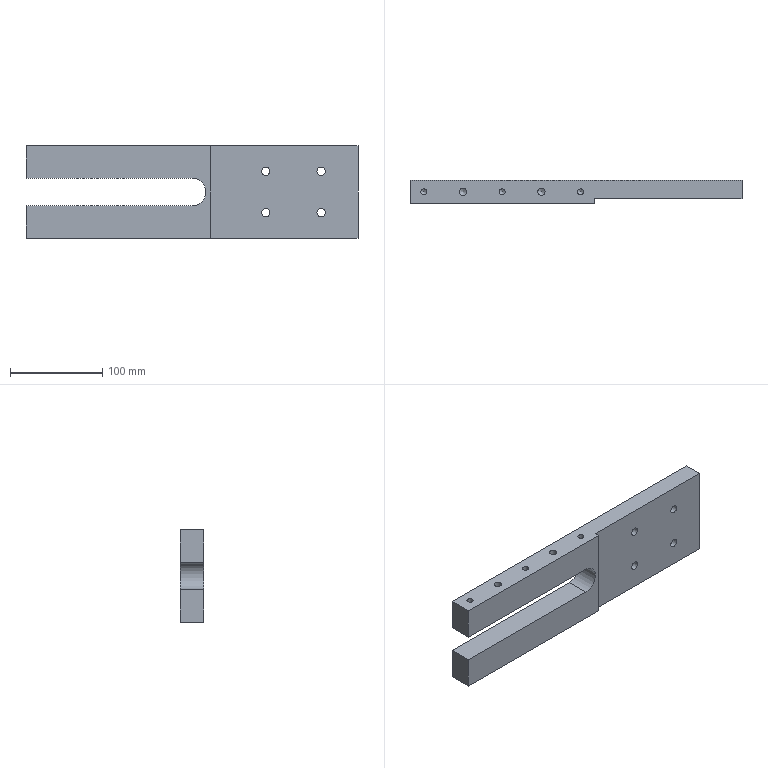Part | STEP file | SN10_003_004_PLACA | 1 solid | 40 faces | box 360 x 25 x 100 mm | volume 661169 mm3 | cylinder 17 | cone 12 | plane 11 | commonest cylinder face diameters 6.647 x8 8 x4 9 x4 30 x1